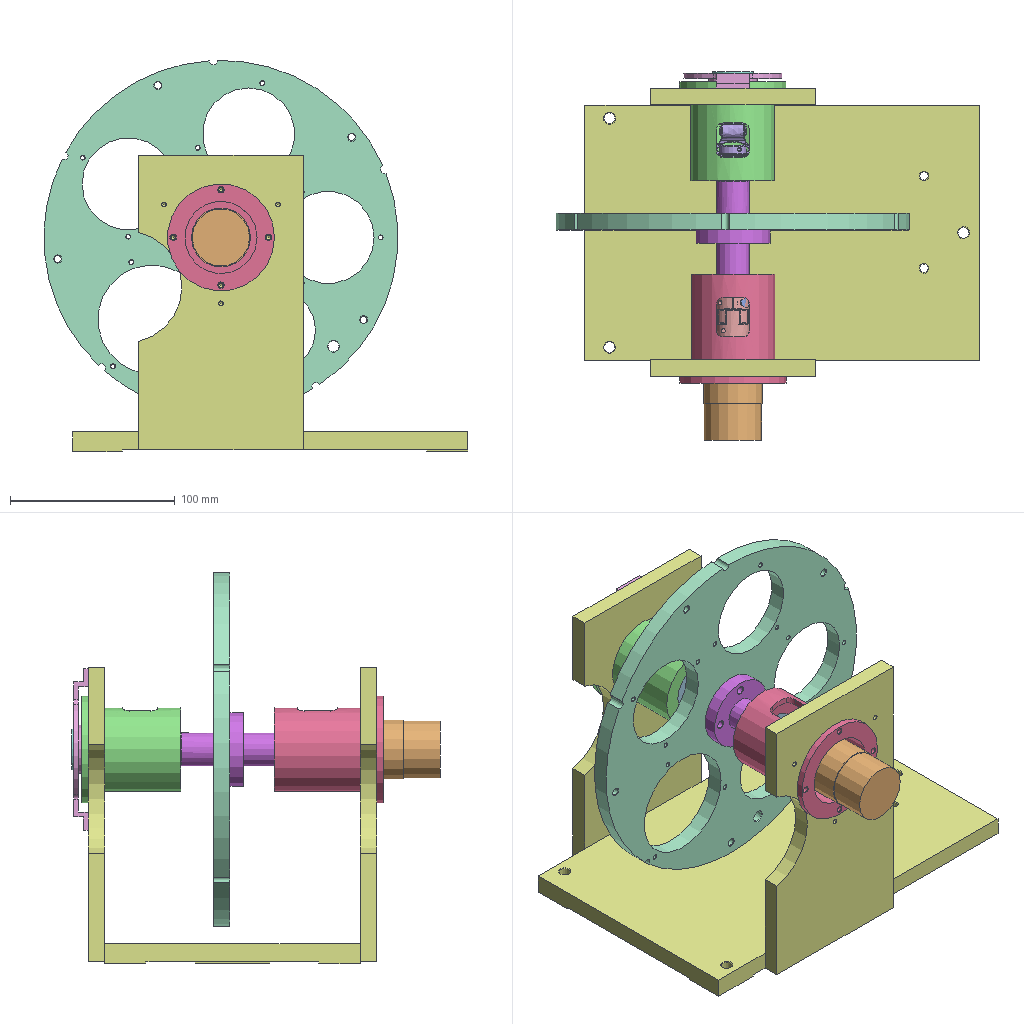Assembly | NX | 11 different items | 12 placed | box 257 x 224 x 237 mm
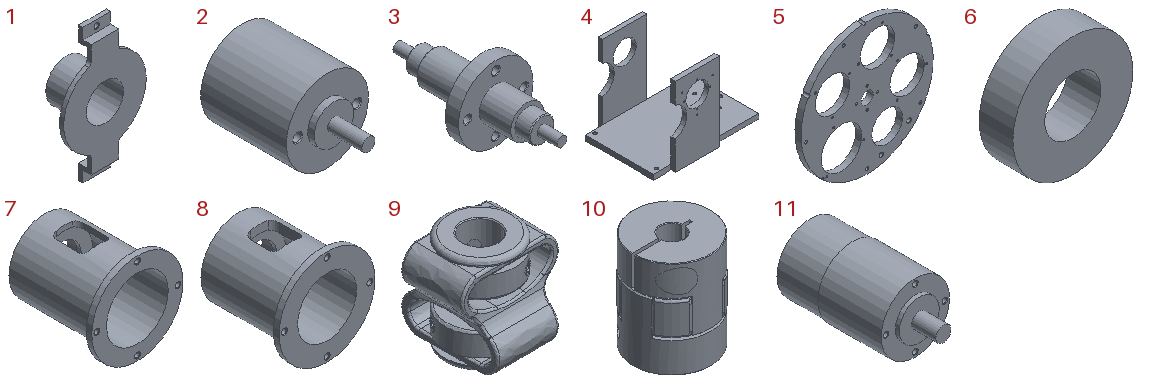Parts list (item | quantity | size | volume | features):
1 | x1 | 60 x 28 x 98 mm | 14363 mm3 | features DATUM_CSYS 8, SKETCH 7, EXTRUDE 5, CSUNK_HOLE 2, HOLE PACKAGE 2, SIMPLE HOLE 2, BLEND 1
2 | x1 | 25 x 38.5 x 25 mm | 13059 mm3 | features DATUM_CSYS 5, SKETCH 4, EXTRUDE 3, SIMPLE HOLE 2, SYMBOLIC_THREAD 2, HOLE PACKAGE 1
3 | x1 | 45 x 99 x 45 mm | 31439 mm3 | features DATUM_CSYS 9, SKETCH 8, EXTRUDE 7, SIMPLE HOLE 4, CHAMFER 1, HOLE PACKAGE 1
4 | x1 | 240 x 175 x 180 mm | 699154 mm3 | features SIMPLE HOLE 18, SYMBOLIC_THREAD 15, DATUM_CSYS 12, SKETCH 11, HOLE PACKAGE 6, EXTRUDE 5
5 | x1 | 215 x 10 x 215 mm | 229405 mm3 | features SIMPLE HOLE 23, SYMBOLIC_THREAD 21, DATUM_CSYS 8, SKETCH 7, HOLE PACKAGE 4, EXTRUDE 3
6 | x2 | 32 x 9 x 32 mm | 5648 mm3 | features DATUM_CSYS 2, EXTRUDE 1, SKETCH 1
7 | x1 | 65 x 66 x 65 mm | 46902 mm3 | features DATUM_CSYS 7, SKETCH 6, EXTRUDE 5, SIMPLE HOLE 4, BLEND 1, HOLE PACKAGE 1
8 | x1 | 65 x 60 x 65 mm | 55807 mm3 | features DATUM_CSYS 7, SKETCH 6, EXTRUDE 5, SIMPLE HOLE 4, BLEND 1, HOLE PACKAGE 1
9 | x1 | 22.041 x 22.041 x 21.943 mm | 3971 mm3 | features BREP 1
10 | x1 | 20 x 20 x 25 mm | 6872 mm3 | features BREP 1
11 | x1 | 36 x 70.2 x 36 mm | 56405 mm3 | features DATUM_CSYS 6, SKETCH 5, EXTRUDE 4, SIMPLE HOLE 4, SYMBOLIC_THREAD 4, HOLE PACKAGE 1
Mates (type | each side: item.copy, entity, surface, feature):
Touch | 6.1 face plane Extrude(1) | 3.1 face plane Extrude(4)
Touch | 3.1 face plane Extrude(2) | 5.1 face plane Extrude(1)
Touch | 4.1 face cylinder Extrude(2) | 3.1 face cylinder Extrude(1)
Touch | 5.1 face cylinder Extrude(2) | 3.1 face cylinder Extrude(1)
Fix | 4.1 component
Touch | 6.1 face plane Extrude(1) | 3.1 face plane Extrude(1)
Touch | 7.1 face cylinder Extrude(1) | 3.1 face cylinder Extrude(5)
Touch | 7.1 face plane Extrude(1) | 4.1 face plane Extrude(1)
Touch | 8.1 face cylinder Extrude(2) | 3.1 face cylinder Extrude(3)
Touch | 9.1 face cylinder Body(1) | 2.1 face cylinder Extrude(3)
Touch | 9.1 face plane Body(1) | 2.1 face plane Extrude(3)
Touch | 1.1 face cylinder Extrude(1) | 2.1 face cylinder Extrude(3)
Touch | 1.1 face plane Extrude(1) | 2.1 face plane Extrude(1)
Touch | 6.1 face plane Extrude(1) | 7.1 face plane Extrude(3)
Touch | 8.1 face plane Extrude(3) | 6.1 face plane Extrude(1)
Touch | 9.1 face cylinder Body(1) | 3.1 face cylinder Extrude(8)
Touch | 10.1 face cylinder Body(1) | 11.1 face cylinder Extrude(4)
Touch | 10.1 face plane Body(1) | 11.1 face plane Extrude(4)
Touch | 3.1 face cylinder Extrude(7) | 10.1 face cylinder Body(1)
Touch | 10.1 face plane Body(1) | 3.1 face plane Extrude(7)
Distance | 2.1 face plane Extrude(3) | 3.1 face plane Extrude(8)